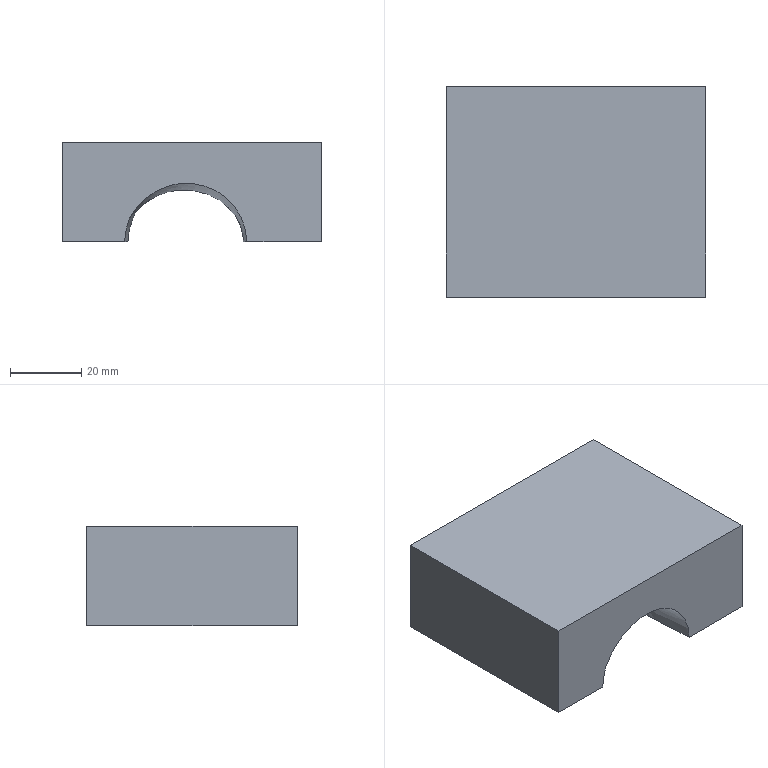NC program | NX | posted with a generic post | part box 72.744 x 59.015 x 27.972 mm
Lines 1 to 1005 of 95982:
N10 G17 G21 G94 G90
(FLOOR_WALL_COPY_1 , TOOL : D63)
N12 T03 M6
N14 G54
N16 G17 G0 G90 X70.872 Y0. S6500 M3
N18 G43 Z30. H3
N20 Z10.025
N22 G94 G1 Z7.025 F1500.
N24 X67.872
N26 X-67.872
N28 X-70.872
N30 Z10.025
N32 G0 Z30.
N34 X70.872
N36 Z9.05
N38 G1 Z6.05
N40 X67.872
N42 X-67.872
N44 X-70.872
N46 Z9.05
N48 G0 Z30.
N50 X70.872
N52 Z8.075
N54 G1 Z5.075
N56 X67.872
N58 X-67.872
N60 X-70.872
N62 Z8.075
N64 G0 Z30.
N66 X70.872
N68 Z7.1
N70 G1 Z4.1
N72 X67.872
N74 X-67.872
N76 X-70.872
N78 Z7.1
N80 G0 Z30.
N82 X70.872
N84 Z6.125
N86 G1 Z3.125
N88 X67.872
N90 X-67.872
N92 X-70.872
N94 Z6.125
N96 G0 Z30.
N98 X70.872
N100 Z5.15
N102 G1 Z2.15
N104 X67.872
N106 X-67.872
N108 X-70.872
N110 Z5.15
N112 G0 Z30.
N114 X70.872
N116 Z4.175
N118 G1 Z1.175
N120 X67.872
N122 X-67.872
N124 X-70.872
N126 Z4.175
N128 G0 Z30.
N130 X70.872
N132 Z3.2
N134 G1 Z0.2
N136 X67.872
N138 X-67.872
N140 X-70.872
N142 Z3.2
N144 G0 Z30.
(FLOOR_WALL_COPY , TOOL : D63)
N146 X70.872
N148 Z3.
N150 G1 Z0.
N152 X67.872
N154 X-67.872
N156 X-70.872
N158 Z3.
N160 G0 Z30.
N162 M5
(DRILLING , TOOL : D6A45)
N164 T01 M6
N166 G54
N168 G17 G0 G90 X-25.98 Y-17.007 S5000 M3
N170 G43 Z30. H1
N172 G94 G81 G98 Z-1. F250. R3.
N174 Y0.
N176 X22.701 Y1.319
N178 X22.872 Y18.771
N180 G80
N182 G0 X22.872 Y18.771 Z30.
N184 M5
(DRILLING_COPY_COPY , TOOL : 4.2ZT)
N186 T13 M6
N188 G54
N190 G17 G0 G90 X-25.98 Y0. S2000 M3
N192 G43 Z30. H13
N194 G94 G83 G98 Z-16.262 F150. Q3. R3.
N196 X22.701 Y1.319
N198 G80
N200 G0 X22.701 Y1.319 Z30.
N202 M5
(DRILLING_COPY_COPY_1 , TOOL : 6.0ZT)
N204 T12 M6
N206 G54
N208 G17 G0 G90 X-25.98 Y-17.007 S2000 M3
N210 G43 Z30. H12
N212 G94 G83 G98 Z-6.803 F150. Q3. R3.
N214 X22.872 Y18.771
N216 G80
N218 G0 X22.872 Y18.771 Z30.
N220 M5
(ZLEVEL_PROFILE , TOOL : D10)
N222 T04 M6
N224 G54
N226 G17 G0 G90 X6.339 Y-35.446 S9500 M3
N228 G43 Z30. H4
N230 Z2.351
N232 G94 G1 Z-0.649 F1000.
N234 X8.783 Y-34.579
N236 G3 X9.432 Y-33.819 R1.
N238 G1 X9.594 Y-32.943 F3000.
N240 X10.353 Y-29.113
N242 G3 X11.174 Y-18.732 R44.736
N244 X10.465 Y-9.092 R135.523
N246 G2 X9.528 Y0.91 R325.209
N248 X9.411 Y14.759 R121.644
N250 X9.859 Y23.223 R452.887
N252 G3 X10.376 Y33.994 R414.056
N254 G1 X10.437 Y35.119
N256 X10.397 Y35.16 Z-1.296
N258 G3 X9.995 Y26.3 R1988.526
N260 X9.326 Y13.99 R418.562
N262 G1 X9.298 Y13.22
N264 G3 X9.504 Y0.141 R115.066
N266 X10.494 Y-9.861 R514.132
N268 G2 X11.135 Y-19.094 R125.7
N270 G1 X11.125 Y-22.179
N272 X11.06 Y-22.941
N274 X11.04 Y-23.711
N276 G2 X10.353 Y-28.93 R42.268
N278 G1 X10.307 Y-29.096
N280 X9.408 Y-33.713
N282 X9.389 Y-33.837
N284 X9.311 Y-33.854 Z-1.939
N286 G2 X10.227 Y-29.204 R167.152
N288 G3 X10.972 Y-23.545 R36.684
N290 X10.881 Y-15.254 R65.015
N292 X10.081 Y-6.784 R218.471
N294 G2 X9.224 Y3.218 R189.269
N296 X9.355 Y17.067 R140.941
N298 G1 X10.072 Y29.378
N300 X10.303 Y34.764
N302 X10.335 Y35.193
N304 X10.293 Y35.197 Z-2.258
N306 X10.242 Y35.201 Z-2.577
N308 X9.894 Y27.839
N310 G3 X9.149 Y15.206 R1037.494
N312 X9.542 Y-2.502 R118.13
N314 X10.353 Y-10.286 R592.303
N316 G2 X10.949 Y-18.325 R129.413
N318 X10.353 Y-28.077 R46.878
N320 G1 X9.202 Y-33.865
N322 X9.078 Y-33.873 Z-3.208
N324 X9.101 Y-33.713
N326 X10.353 Y-27.445
N328 G3 X10.858 Y-19.094 R46.636
N330 X10.247 Y-10.631 R108.014
N332 G2 X9.329 Y-1.836 R626.712
N334 X8.876 Y11.93 R107.709
N336 X9.374 Y21.684 R238.756
N338 G1 X9.408 Y22.453
N340 X9.475 Y23.223
N342 G3 X10.139 Y35.21 R724.458
N344 G1 X10.06 Y35.216 Z-3.519
N346 X9.995 Y35.221 Z-3.831
N348 G2 X9.312 Y23.223 R809.16
N350 G1 X9.256 Y22.453
N352 G3 X8.717 Y12.777 R318.099
N354 X9.068 Y-0.87 R103.127
N356 G1 X9.4 Y-4.476
N358 G2 X10.366 Y-13.394 R340.168
N360 X10.735 Y-20.556 R82.791
N362 X9.905 Y-29.054 R40.595
N364 G1 X8.948 Y-33.713
N366 X8.925 Y-33.876
N368 X8.851 Y-33.877 Z-4.137
N370 X8.765 Z-4.444
N372 X8.939 Y-32.943
N374 X9.732 Y-29.111
N376 G3 X10.573 Y-19.114 R41.802
N378 X10.006 Y-11.4 R104.84
N380 X9.357 Y-5.659 R763.831
N382 G2 X8.546 Y3.218 R176.621
N384 X8.675 Y16.298 R119.75
N386 G1 X8.725 Y17.067
N388 G2 X9.066 Y22.453 R731.199
N390 G1 X9.133 Y23.223
N392 G3 X9.821 Y35.234 R541.045
N394 G1 X9.733 Y35.241 Z-4.743
N396 X9.642 Y35.248 Z-5.043
N398 X9.2 Y27.07
N400 G3 X8.39 Y15.529 R662.276
N402 X8.309 Y3.218 R119.617
N404 X9.364 Y-7.553 R184.128
N406 G2 X10.32 Y-17.555 R149.783
N408 X9.857 Y-27.558 R44.712
N410 G1 X9.712 Y-28.327
N412 X8.57 Y-33.864
N414 X8.468 Y-33.857 Z-5.333
N416 X8.372 Y-33.85 Z-5.623
N418 X9.406 Y-28.901
N420 G3 X10.209 Y-20.64 R38.185
N422 X9.679 Y-12.17 R84.12
N424 G1 X8.767 Y-4.476
N426 X8.666 Y-3.706
N428 X8.571 Y-2.937
N430 X8.506 Y-2.167
N432 X8.263 Y0.455
N434 G2 X7.922 Y8.211 R79.981
N436 X8.46 Y20.145 R147.996
N438 X8.676 Y23.223 R120.911
N440 G1 X8.809 Y24.736
N442 G3 X9.445 Y35.26 R464.927
N444 G1 X9.34 Y35.266 Z-5.907
N446 X9.238 Y35.272 Z-6.192
N448 X8.809 Y28.019
N450 X8.74 Y27.07
N452 G3 X7.848 Y15.529 R583.08
N454 X7.706 Y3.988 R103.887
N456 X8.883 Y-7.553 R148.977
N458 G2 X9.957 Y-18.325 R143.175
N460 X9.453 Y-27.558 R41.597
N462 G1 X9.31 Y-28.327
N464 X8.166 Y-33.713
N466 X8.148 Y-33.831
N468 X8.03 Y-33.823 Z-6.473
N470 X7.902 Y-33.815 Z-6.753
N472 X9.226 Y-27.558
N474 G3 X9.744 Y-19.094 R39.432
N476 X8.807 Y-9.092 R109.813
N478 G2 X7.752 Y-0.629 R274.239
N480 G1 X7.425 Y3.218
N482 G2 X7.536 Y15.529 R107.691
N484 X8.475 Y27.07 R660.147
N486 G3 X9. Y35.286 R752.635
N488 G1 X8.882 Y35.293 Z-7.026
N490 X8.749 Y35.301 Z-7.298
N492 G3 X8.426 Y30.147 R118.708
N494 G1 X8.373 Y29.378
N496 X8.037 Y25.2
N498 G3 X7.112 Y13.99 R282.241
N500 X7.414 Y-0.629 R87.771
N502 G1 X7.511 Y-1.398
N504 X7.587 Y-2.167
N506 X8.855 Y-11.763
N508 G2 X9.52 Y-19.692 R83.246
N510 X8.677 Y-29.036 R37.363
N512 G1 X7.651 Y-33.713
N514 X7.637 Y-33.799
N516 X7.491 Y-33.788 Z-7.559
N518 X7.35 Y-33.778 Z-7.821
N520 X7.36 Y-33.713
N522 X8.714 Y-27.558
N524 X8.809 Y-27.066
N526 G3 X9.163 Y-17.555 R41.263
N528 X7.876 Y-6.784 R161.755
N530 G2 X6.719 Y3.218 R129.688
N532 X7.054 Y18.36 R106.4
N534 G1 X8.085 Y29.378
N536 X8.428 Y34.764
N538 X8.47 Y35.32
N540 X8.353 Y35.327 Z-8.072
N542 X8.201 Y35.337 Z-8.324
N544 G2 X7.265 Y23.864 R343.965
N546 G1 X7.189 Y23.223
N548 G3 X6.295 Y12.425 R168.551
N550 X7.007 Y-3.016 R80.444
N552 G1 X7.767 Y-8.323
N554 X7.884 Y-9.092
N556 G2 X8.968 Y-19.094 R105.46
N558 X8.037 Y-29.437 R35.63
N560 G1 X7.043 Y-33.755
N562 X6.898 Y-33.744 Z-8.567
N564 X6.734 Y-33.732 Z-8.81
N566 X6.913 Y-32.943
N568 X7.821 Y-29.119
N570 G3 X8.675 Y-19.034 R34.177
N572 X7.434 Y-8.323 R105.355
N574 G2 X6.225 Y0.141 R210.374
N576 X6.073 Y15.529 R79.197
N578 X7.265 Y27.102 R385.695
N580 G1 X7.92 Y35.357
N582 X7.783 Y35.367 Z-9.045
N584 X7.615 Y35.379 Z-9.279
N586 G2 X6.493 Y23.391 R246.453
N588 G3 X5.521 Y13.627 R212.909
N590 X5.762 Y0.726 R68.149
N592 G1 X6.004 Y-1.398
N594 X6.957 Y-7.553
N596 X7.353 Y-9.957
N598 G2 X8.391 Y-19.283 R89.956
N600 X7.867 Y-27.558 R34.08
N602 G1 X6.426 Y-33.708
N604 X6.264 Y-33.693 Z-9.504
N606 X6.089 Y-33.677 Z-9.73
N608 X7.405 Y-28.327
N610 G3 X8.092 Y-19.094 R32.734
N612 X6.595 Y-7.553 R105.795
N614 G2 X5.324 Y0.801 R124.203
N616 X5.254 Y15.803 R67.015
N618 G1 X5.64 Y19.376
N620 X6.493 Y26.439
N622 X6.56 Y27.07
N624 X7.322 Y35.4
N626 X7.169 Y35.411 Z-9.945
N628 X7.001 Y35.424 Z-10.161
N630 G2 X5.205 Y19.376 R277.244
N632 G3 X4.544 Y3.988 R79.68
N634 X6.346 Y-8.323 R123.906
N636 G2 X7.784 Y-19.094 R87.154
N638 X7.265 Y-27.595 R32.942
N640 G1 X5.765 Y-33.648
N642 X5.598 Y-33.63 Z-10.368
N644 X5.42 Y-33.611 Z-10.574
N646 X6.946 Y-27.558
N648 X7.102 Y-26.788
N650 G3 X7.367 Y-17.555 R34.192
N652 X5.721 Y-6.993 R115.46
N654 G2 X3.975 Y5.526 R93.648
N656 X4.767 Y19.376 R78.342
N658 G3 X6.684 Y35.449 R255.827
N660 G1 X6.537 Y35.46 Z-10.77
N662 X6.367 Y35.474 Z-10.966
N664 G2 X4.539 Y20.914 R207.585
N666 G3 X3.427 Y7.065 R83.088
N668 X4.964 Y-5.245 R72.463
N670 G2 X7.046 Y-17.555 R127.058
N672 X6.493 Y-28.208 R31.215
N674 G1 X6.247 Y-29.096
N676 X5.085 Y-33.576
N678 X4.924 Y-33.558 Z-11.152
N680 X4.733 Y-33.537 Z-11.338
N682 X6.317 Y-27.558
N684 X6.488 Y-26.788
N686 G3 X6.546 Y-16.017 R34.38
N688 X4.377 Y-4.476 R157.772
N690 G2 X2.879 Y7.835 R67.81
N692 X3.986 Y20.129 R79.387
N694 G3 X6.038 Y35.502 R222.23
N696 G1 X5.888 Y35.515 Z-11.514
N698 X5.727 Y35.529 Z-11.69
N700 G2 X3.528 Y20.145 R220.724
N702 G3 X2.363 Y7.065 R68.177
N704 X4.109 Y-5.245 R65.438
N706 G2 X6.415 Y-17.555 R120.012
N708 X5.999 Y-27.558 R29.773
N710 G1 X5.818 Y-28.327
N712 X4.375 Y-33.498
N714 X4.202 Y-33.478 Z-11.856
N716 X4.02 Y-33.457 Z-12.022
N718 X5.491 Y-28.327
N720 X5.721 Y-27.447
N722 G3 X5.897 Y-16.017 R31.355
N724 X3.406 Y-4.037 R170.523
N726 G2 X2.546 Y17.067 R51.388
N728 G1 X3.917 Y24.971
N730 G3 X5.397 Y35.56 R162.542
N732 G1 X5.248 Y35.574 Z-12.177
N734 X5.084 Y35.59 Z-12.332
N736 G2 X2.573 Y20.145 R174.001
N738 G3 X1.252 Y7.065 R61.632
N740 X3.052 Y-4.476 R61.71
N742 G2 X5.582 Y-16.017 R138.209
N744 X5.553 Y-26.788 R30.899
N746 G1 X5.372 Y-27.558
N748 X3.668 Y-33.413
N750 X3.502 Y-33.391 Z-12.477
N752 X3.33 Y-33.368 Z-12.621
N754 X4.95 Y-28.028
N756 X5.071 Y-27.558
N758 G3 X5.373 Y-16.786 R27.306
N760 X2.804 Y-5.245 R100.196
N762 G2 X0.769 Y5.526 R64.023
N764 X1.948 Y19.376 R49.723
N766 G3 X4.772 Y35.621 R170.733
N768 G1 X4.629 Y35.636 Z-12.755
N770 X4.47 Y35.653 Z-12.889
N772 X3.406 Y28.55
N774 X3.121 Y27.07
N776 X1.309 Y18.606
N778 X0.776 Y15.828
N780 G3 X1.16 Y-0.316 R38.114
N782 G1 X1.98 Y-3.706
N784 G2 X4.95 Y-15.901 R148.998
N786 X4.968 Y-26.788 R29.66
N788 G1 X4.773 Y-27.558
N790 X2.989 Y-33.318
N792 X2.833 Y-33.294 Z-13.011
N794 X2.668 Y-33.268 Z-13.134
N796 X4.487 Y-27.558
N798 X4.682 Y-26.788
N800 G3 X4.665 Y-16.017 R27.403
N802 X1.738 Y-4.476 R110.213
N804 G2 X-0.494 Y7.065 R54.271
N806 X0.972 Y19.376 R44.729
N808 G3 X4.188 Y35.684 R146.131
N810 G1 X4.045 Y35.701 Z-13.246
N812 X3.908 Y35.717 Z-13.357
N814 G2 X0.483 Y19.376 R129.167
N816 G3 X-0.877 Y4.757 R38.621
N818 X1.332 Y-4.476 R59.136
N820 G2 X4.508 Y-16.786 R96.652
N822 X4.225 Y-27.558 R24.937
N824 G1 X3.987 Y-28.327
N826 X2.358 Y-33.215
N828 X2.213 Y-33.189 Z-13.458
N830 X2.069 Y-33.164 Z-13.558
N832 X3.967 Y-27.558
N834 X4.181 Y-26.788
N836 G3 X4.178 Y-16.291 R26.3
N838 X1.09 Y-4.962 R94.501
N840 G1 X-0.194 Y-0.823
N842 G2 X-1.741 Y9.373 R34.478
N844 X0.318 Y20.526 R51.448
N846 G3 X3.651 Y35.748 R107.634
N848 X3.279 Y36.676 R1.
N850 G1 X1.293 Y38.24
N852 Z-10.558
N854 G0 Z30.
N856 X-12.168 Y38.156
N858 Z2.351
N860 G1 Z-0.649 F1000.
N862 X-14.167 Y36.537
N864 G3 X-14.526 Y35.603 R1.
N866 G2 X-13.502 Y28.608 R296.97 F3000.
N868 X-13.329 Y7.835 R83.197
N870 G3 X-13.417 Y4.757 R14.398
N872 G2 X-15.223 Y-18.596 R84.348
N874 G3 X-15.284 Y-19.199 R2.628
N876 X-14.237 Y-29.096 R55.047
N878 G1 X-13.309 Y-33.816
N880 X-13.255 Y-33.839 Z-1.296
N882 X-13.876 Y-30.635
N884 X-14.035 Y-29.866
N886 G2 X-15.247 Y-19.094 R56.765
N888 G1 X-15.209 Y-18.707
N890 G3 X-13.324 Y3.988 R83.761
N892 G1 X-13.381 Y4.988
N894 G2 X-13.265 Y8.162 R17.013
N896 G3 X-12.983 Y10.856 R53.59
N898 X-13.266 Y27.07 R83.968
N900 X-14.495 Y35.622 R278.481
N902 G1 X-14.442 Y35.647 Z-1.939
N904 G2 X-13.431 Y28.889 R301.166
N906 X-13.26 Y7.435 R83.172
N908 G3 X-13.32 Y5.203 R11.819
N910 G2 X-15.12 Y-18.616 R83.665
N912 G3 X-15.178 Y-19.181 R2.433
N914 X-14.13 Y-29.063 R55.059
N916 G1 X-13.178 Y-33.857
N918 X-13.087 Y-33.869 Z-2.577
N920 X-13.11 Y-33.713
N922 X-14.049 Y-29.013
N924 G2 X-15.081 Y-19.178 R53.468
N926 X-15.017 Y-18.567 R2.664
N928 G3 X-13.158 Y3.988 R82.976
N930 G1 X-13.219 Y5.106
N932 G2 X-13.134 Y7.763 R15.413
N934 G3 X-13.308 Y28.608 R82.477
N936 X-14.37 Y35.675 R236.416
N938 G1 X-14.25 Y35.637 Z-3.208
N940 G2 X-13.271 Y29.167 R366.336
N942 X-12.917 Y8.604 R83.095
N944 G1 X-13.088 Y7.065
N946 G3 X-13.125 Y5.526 R8.739
N948 G2 X-14.921 Y-18.594 R82.052
N950 G3 X-14.974 Y-19.075 R2.154
N952 X-13.91 Y-29.096 R49.119
N954 G1 X-12.955 Y-33.877
N956 X-12.887 Y-33.88 Z-3.519
N958 X-12.812 Y-33.883 Z-3.831
N960 X-12.841 Y-33.713
N962 X-13.761 Y-29.096
N964 X-13.939 Y-28.327
N966 G2 X-14.849 Y-19.257 R55.662
N968 X-14.776 Y-18.544 R2.987
N970 G3 X-12.883 Y3.988 R81.829
N972 G1 X-12.97 Y5.526
N974 G2 X-12.874 Y7.835 R13.275
N976 G3 X-13.058 Y28.608 R82.135
N978 X-14.125 Y35.582 R267.853
N980 G1 X-13.952 Y35.538 Z-4.444
N982 G2 X-12.822 Y27.91 R240.627
N984 X-12.749 Y7.642 R79.674
N986 G3 X-12.819 Y5.526 R11.621
N988 G2 X-14.656 Y-18.691 R81.455
N990 G1 X-14.717 Y-19.094
N992 X-14.686 Y-19.864
N994 X-14.582 Y-22.172
N996 X-14.497 Y-22.941
N998 X-14.482 Y-23.149
N1000 G3 X-13.756 Y-28.421 R41.633
N1002 G1 X-12.645 Y-33.876
N1004 X-12.554 Y-33.871 Z-4.743
N1006 X-12.467 Y-33.866 Z-5.043
N1008 X-12.491 Y-33.713
N1010 X-13.507 Y-28.788
N1012 G2 X-14.479 Y-20.619 R48.434
N1014 G1 X-14.519 Y-19.425
N1016 G2 X-14.419 Y-18.376 R4.114
N1018 G3 X-12.583 Y4.757 R80.753
N1020 G1 X-12.628 Y5.526
N1022 G2 X-12.549 Y7.835 R11.821
N1024 G3 X-12.629 Y27.839 R82.372
N1026 G2 X-13.613 Y35.294 R160.842
N1028 G1 X-13.453 Y35.283 Z-5.333
N1030 X-13.29 Y35.272 Z-5.623
N1032 X-12.999 Y31.686
N1034 X-12.896 Y30.917
N1036 X-12.452 Y27.839
N1038 X-12.36 Y27.07
N1040 G2 X-12.371 Y7.835 R79.771
N1042 G3 X-12.44 Y5.526 R11.863
N1044 G2 X-14.348 Y-18.821 R79.515
N1046 G3 X-13.559 Y-27.558 R53.953
N1048 G1 X-12.258 Y-33.852
N1050 X-12.143 Y-33.842 Z-5.907
N1052 X-12.025 Y-33.833 Z-6.192
N1054 X-13.166 Y-28.425
N1056 G2 X-14.049 Y-21.399 R42.692
N1058 G1 X-14.156 Y-18.848
N1060 G3 X-12.221 Y5.526 R79.349
N1062 G2 X-12.167 Y7.835 R10.804
N1064 G3 X-12.597 Y30.147 R79.745
N1066 G1 X-12.669 Y30.917
N1068 X-12.976 Y35.285
N1070 X-12.817 Y35.291 Z-6.473
N1072 X-12.664 Y35.298 Z-6.753
N1074 X-12.622 Y34.764
N1076 X-12.336 Y30.147
N1078 X-12.261 Y29.378
N1080 G2 X-11.958 Y7.835 R78.674
N1082 G3 X-11.997 Y5.526 R11.438
N1084 G2 X-13.576 Y-17.227 R76.997
N1086 G1 X-13.902 Y-18.681
N1088 X-13.92 Y-18.874
N1090 G3 X-12.832 Y-28.914 R48.229
N1092 G1 X-11.772 Y-33.818
N1094 X-11.641 Y-33.81 Z-7.026
N1096 X-11.506 Y-33.801 Z-7.298
N1098 X-11.52 Y-33.713
N1100 X-12.804 Y-27.879
N1102 G2 X-13.689 Y-18.704 R49.902
N1104 G3 X-12.032 Y-9.369 R73.392
N1106 X-11.755 Y5.526 R72.103
N1108 G2 X-11.473 Y10.143 R71.719
N1110 G3 X-11.13 Y18.606 R85.202
N1112 X-11.912 Y28.608 R85.687
N1114 G1 X-12.36 Y35.31
N1116 X-12.211 Y35.317 Z-7.559
N1118 X-12.069 Y35.323 Z-7.821
N1120 X-11.532 Y27.839
N1122 X-11.465 Y27.07
N1124 X-11.243 Y24.815
N1126 G2 X-10.932 Y15.027 R73.707
N1128 G1 X-10.994 Y13.22
N1130 X-11.443 Y4.907
N1132 X-11.442 Y4.757
N1134 G2 X-13.442 Y-18.645 R76.004
N1136 G1 X-13.421 Y-19.094
N1138 X-13.359 Y-20.936
N1140 G3 X-12.259 Y-29.145 R41.6
N1142 G2 X-11.231 Y-33.781 R161.339
N1144 G1 X-11.083 Y-33.769 Z-8.072
N1146 X-10.922 Y-33.756 Z-8.324
N1148 X-11.803 Y-29.866
N1150 X-11.882 Y-29.551
N1152 G2 X-13.111 Y-20.541 R41.394
N1154 G1 X-13.148 Y-19.094
N1156 X-13.164 Y-18.677
N1158 X-13.112 Y-18.325
N1160 X-12.786 Y-16.855
N1162 G3 X-11.129 Y3.988 R75.557
N1164 X-10.742 Y21.684 R132.674
N1166 X-11.768 Y35.355 R1114.465
N1168 G1 X-11.63 Y35.371 Z-8.567
N1170 X-11.474 Y35.39 Z-8.81
N1172 G3 X-10.678 Y26.3 R1104.06
N1174 G2 X-10.815 Y3.218 R121.382
N1176 X-12.88 Y-18.325 R75.214
N1178 G3 X-11.748 Y-28.92 R43.315
N1180 G1 X-10.622 Y-33.731
N1182 X-10.472 Y-33.718 Z-9.045
N1184 X-10.311 Y-33.704 Z-9.279
N1186 X-11.501 Y-28.709
N1188 G2 X-12.549 Y-20.675 R38.964
N1190 G1 X-12.609 Y-18.325
N1192 X-12.549 Y-17.988
N1194 G3 X-10.474 Y-0.19 R73.57
N1196 G1 X-10.49 Y2.449
N1198 G3 X-10.101 Y23.992 R108.574
N1200 G1 X-10.221 Y25.531
N1202 X-11.176 Y35.424
N1204 X-11.024 Y35.442 Z-9.504
N1206 X-10.85 Y35.462 Z-9.73
N1208 X-9.83 Y25.531
N1210 G2 X-10.084 Y2.015 R103.008
N1212 G3 X-10.187 Y0.251 R13.157
N1214 G2 X-12.29 Y-17.935 R73.854
N1216 G3 X-11.295 Y-28.327 R42.45
N1218 G1 X-9.987 Y-33.672
N1220 X-9.829 Y-33.656 Z-9.945
N1222 X-9.666 Y-33.64 Z-10.161
N1224 X-10.974 Y-28.327
N1226 G2 X-11.997 Y-19.094 R38.829
N1228 X-11.873 Y-17.232 R5.344
N1230 G1 X-11.763 Y-16.786
N1232 G3 X-9.995 Y-3.908 R73.119
N1234 X-9.891 Y0.141 R92.621
N1236 X-9.206 Y23.223 R98.449
N1238 X-10.537 Y35.498 R636.712
N1240 G1 X-10.377 Y35.516 Z-10.368
N1242 X-10.215 Y35.534 Z-10.574
N1244 X-9.095 Y26.3
N1246 X-8.765 Y23.091
N1248 G2 X-9.573 Y-0.629 R87.193
N1250 G3 X-9.713 Y-3.581 R317.09
N1252 G2 X-11.689 Y-17.555 R72.48
N1254 G3 X-11.276 Y-25.249 R48.498
N1256 X-10.5 Y-28.954 R41.757
N1258 G1 X-9.304 Y-33.608
N1260 X-9.136 Y-33.593 Z-10.77
N1262 X-8.958 Y-33.577 Z-10.966
N1264 X-10.488 Y-27.736
N1266 G2 X-11.365 Y-17.201 R40.276
N1268 G3 X-9.758 Y-7.794 R68.528
N1270 X-9.355 Y-2.167 R100.065
N1272 X-8.323 Y23.223 R84.73
N1274 G1 X-8.495 Y24.761
N1276 X-9.881 Y35.571
N1278 X-9.72 Y35.589 Z-11.152
N1280 X-9.548 Y35.608 Z-11.338
N1282 X-8.061 Y24.761
N1284 X-7.796 Y22.453
N1286 G2 X-8.499 Y0.141 R75.903
N1288 G1 X-8.62 Y-0.629
N1290 X-8.987 Y-2.529
N1292 G3 X-9.22 Y-4.411 R14.016
N1294 G2 X-11.023 Y-16.786 R70.105
N1296 G3 X-9.716 Y-29.439 R37.484
N1298 G1 X-9.596 Y-29.866
N1300 X-9.385 Y-30.635
N1302 X-8.596 Y-33.539
N1304 X-8.432 Y-33.522 Z-11.514
N1306 X-8.25 Y-33.502 Z-11.69
N1308 X-9.469 Y-29.096
N1310 X-9.716 Y-28.267
N1312 G2 X-10.607 Y-16.017 R35.54
N1314 G3 X-9.229 Y-7.605 R65.078
N1316 G1 X-9. Y-5.245
N1318 X-8.944 Y-4.74
N1320 X-8.159 Y-0.629
N1322 X-7.723 Y1.882
N1324 G3 X-7.222 Y21.389 R67.043
N1326 G1 X-7.63 Y24.761
N1328 X-9.217 Y35.645
N1330 X-9.055 Y35.663 Z-11.856
N1332 X-8.897 Y35.681 Z-12.022
N1334 X-7.084 Y23.992
N1336 X-6.66 Y20.591
N1338 G2 X-7.376 Y0.991 R61.351
N1340 G1 X-8.775 Y-6.014
N1342 G2 X-10.335 Y-16.017 R98.084
N1344 G3 X-9.716 Y-26.988 R37.429
N1346 G1 X-7.893 Y-33.459
N1348 X-7.726 Y-33.437 Z-12.177
N1350 X-7.549 Y-33.415 Z-12.332
N1352 X-9.256 Y-27.558
N1354 X-9.447 Y-26.788
N1356 G2 X-9.945 Y-15.247 R37.022
N1358 G3 X-8.684 Y-7.553 R114.997
N1360 G1 X-8.543 Y-6.784
N1362 X-7.176 Y-0.629
N1364 X-6.69 Y1.83
N1366 G3 X-6.098 Y19.979 R56.196
N1368 G1 X-6.521 Y23.223
N1370 X-8.562 Y35.719
N1372 X-8.403 Y35.737 Z-12.477
N1374 X-8.246 Y35.755 Z-12.621
N1376 X-6.06 Y23.223
N1378 X-5.584 Y19.765
N1380 G2 X-6.74 Y-0.867 R53.944
N1382 G3 X-9.408 Y-13.708 R149.58
N1384 X-9.147 Y-26.788 R35.566
N1386 G1 X-8.962 Y-27.558
N1388 X-7.206 Y-33.367
N1390 X-7.038 Y-33.342 Z-12.755
N1392 X-6.871 Y-33.317 Z-12.889
N1394 X-8.656 Y-27.558
N1396 X-8.861 Y-26.788
N1398 G2 X-9.221 Y-14.478 R35.054
N1400 X-6.241 Y-0.813 R119.511
N1402 G3 X-4.986 Y18.943 R47.529
N1404 G1 X-5.617 Y23.223
N1406 X-7.606 Y33.994
N1408 X-7.93 Y35.793
N1410 X-7.784 Y35.81 Z-13.011
N1412 X-7.633 Y35.829 Z-13.134
N1414 G2 X-4.622 Y20.018 R3728.251
N1416 X-5.345 Y0.711 R43.579
N1418 G1 X-7.124 Y-5.946
N1420 G3 X-8.955 Y-14.745 R80.656
N1422 X-8.741 Y-26.019 R33.611
N1424 X-6.556 Y-33.267 R78.335
N1426 G1 X-6.405 Y-33.24 Z-13.246
N1428 X-6.251 Y-33.212 Z-13.357
N1430 X-7.401 Y-29.769
N1432 X-8.056 Y-27.68
N1434 G2 X-8.953 Y-22.951 R20.676
N1436 X-8.172 Y-11.871 R39.47
N1438 X-5.207 Y-0.629 R147.134
N1440 G3 X-4.037 Y19.376 R40.93
N1442 G1 X-6.988 Y33.994
N1444 X-7.356 Y35.863
N1446 X-7.225 Y35.881 Z-13.458
N1448 X-7.091 Y35.899 Z-13.558
N1450 X-6.629 Y33.554
N1452 X-3.435 Y18.811
N1454 G2 X-3.54 Y3.715 R34.553
N1456 G1 X-3.832 Y2.449
N1458 X-6.816 Y-7.553
N1460 G3 X-8.749 Y-17.886 R55.644
N1462 X-7.467 Y-28.74 R26.467
N1464 G1 X-5.974 Y-33.163
N1466 X-5.843 Y-33.137 Z-13.648
N1468 X-5.703 Y-33.11 Z-13.738
N1470 X-7.401 Y-28.243
N1472 X-7.615 Y-27.558
N1474 G2 X-8.215 Y-15.247 R28.015
N1476 X-4.519 Y-1.398 R79.791
N1478 G3 X-2.299 Y7.434 R43.424
N1480 X-0.115 Y-2.512 R38.112
N1482 G2 X3.707 Y-15.247 R113.623
N1484 X4.11 Y-26.019 R26.494
N1486 X1.805 Y-33.114 R61.292
N1488 G1 X1.659 Y-33.083 Z-13.826
N1490 X1.522 Y-33.052 Z-13.914
N1492 X3.498 Y-27.558
N1494 X3.711 Y-26.788
N1496 G3 X3.772 Y-16.786 R23.497
N1498 X0.318 Y-5.025 R69.677
N1500 G2 X-2.382 Y3.694 R70.435
N1502 G1 X-2.736 Y2.449
N1504 X-5.857 Y-6.585
N1506 G3 X-8.36 Y-19.094 R49.598
N1508 X-6.847 Y-29.096 R24.208
N1510 G1 X-5.413 Y-33.048
N1512 X-5.271 Y-33.018 Z-14.001
N1514 X-5.123 Y-32.987 Z-14.087
N1516 X-6.806 Y-28.561
N1518 G2 X-8.065 Y-22.707 R19.806
N1520 X-6.629 Y-10.315 R35.748
N1522 X-2.476 Y1.364 R132.933
N1524 G1 X0.88 Y-7.553
N1526 G2 X3.663 Y-17.555 R57.291
N1528 X3.481 Y-26.788 R22.669
N1530 G1 X3.252 Y-27.558
N1532 X1.24 Y-32.991
N1534 X1.099 Y-32.957 Z-14.174
N1536 X0.947 Y-32.92 Z-14.261
N1538 X2.994 Y-27.558
N1540 X3.231 Y-26.788
N1542 G3 X3.165 Y-16.215 R23.264
N1544 X-0.775 Y-4.371 R72.939
N1546 G1 X-2.509 Y-0.348
N1548 G3 X-6.985 Y-12.939 R71.232
N1550 X-7.495 Y-25.249 R29.801
N1552 X-4.816 Y-32.915 R47.087
N1554 G1 X-4.661 Y-32.876 Z-14.349
N1556 X-4.499 Y-32.835 Z-14.436
N1558 X-5.92 Y-29.439
N1560 G2 X-7.501 Y-17.447 R23.08
N1562 X-2.502 Y-1.973 R45.804
N1564 X3.002 Y-16.786 R60.231
N1566 X2.969 Y-26.788 R21.531
N1568 G1 X2.634 Y-27.839
N1570 X0.918 Y-32.174
N1572 X0.633 Y-32.834
N1574 X0.483 Y-32.792 Z-14.525
N1576 X0.31 Y-32.744 Z-14.613
N1578 X0.557 Y-32.174
N1580 X2.45 Y-27.558
N1582 X2.704 Y-26.788
N1584 G3 X2.876 Y-17.555 R20.413
N1586 X-2.491 Y-3.336 R48.881
N1588 X-7.401 Y-19.568 R37.6
N1590 X-5.733 Y-29.096 R20.774
N1592 G1 X-4.313 Y-32.442
N1594 X-4.168 Y-32.744
N1596 X-3.998 Y-32.691 Z-14.701
N1598 X-3.823 Y-32.636 Z-14.789
N1600 X-4.04 Y-32.174
N1602 X-5.408 Y-29.096
N1604 G2 X-7.161 Y-20.633 R19.329
N1606 X-2.483 Y-4.581 R32.792
N1608 X2.528 Y-17.203 R42.318
N1610 X2.634 Y-25.967 R21.571
N1612 X-0.046 Y-32.632 R39.521
N1614 G1 X-0.229 Y-32.574 Z-14.876
N1616 X-0.414 Y-32.514 Z-14.964
N1618 G3 X2.517 Y-25.249 R31.013
N1620 X2.129 Y-16.786 R21.031
N1622 G1 X1.944 Y-16.017
N1624 G3 X-2.489 Y-5.828 R34.246
N1626 X-6.858 Y-22.034 R28.69
N1628 X-5.18 Y-28.922 R17.386
N1630 G1 X-3.541 Y-32.366
N1632 X-3.465 Y-32.516
N1634 X-3.27 Y-32.434 Z-15.052
N1636 X-3.077 Y-32.353 Z-15.14
N1638 X-4.712 Y-29.096
N1640 G2 X-6.505 Y-22.941 R16.573
N1642 X-2.483 Y-6.995 R25.686
N1644 X2.411 Y-20.259 R29.149
N1646 X1.531 Y-27.558 R16.235
N1648 G1 X-0.454 Y-31.738
N1650 X-0.8 Y-32.351
N1652 X-0.999 Y-32.263 Z-15.228
N1654 X-1.212 Y-32.169 Z-15.316
N1656 G3 X1.923 Y-25.249 R25.455
N1658 X1.475 Y-16.786 R19.503
N1660 G1 X1.261 Y-16.017
N1662 G3 X-2.467 Y-8.042 R25.492
N1664 X-5.84 Y-25.249 R23.275
N1666 X-2.668 Y-32.174 R28.177
N1668 X-1.782 Y-32.638 R1.
N1670 G1 X-1.937 Y-27.179
N1672 Z-12.316
N1674 G0 Z30.
N1676 X-1.555 Y-18.296
N1678 Z-12.492
N1680 G1 Z-15.492 F1000.
N1682 X1.231 Y-19.624
N1684 G2 X1.797 Y-20.448 R1.
N1686 X1.593 Y-25.249 R19.875 F3000.
N1688 X-1.639 Y-31.915 R21.543
N1690 X-2.253 Y-31.913 R-0.311
N1692 X-5.505 Y-25.249 R23.663
N1694 X-2.459 Y-9.1 R21.422
N1696 X0.318 Y-14.338 R20.416
N1698 X1.797 Y-20.448 R19.875
N1700 G1 X1.645 Y-20.462 Z-15.581
N1702 X1.447 Y-20.481 Z-15.67
N1704 G3 X-2.443 Y-10.182 R20.886
N1706 X-5.169 Y-25.249 R19.728
N1708 X-1.961 Y-31.443 R20.96
N1710 X1.502 Y-23.711 R15.592
N1712 X1.447 Y-20.481 R20.886
N1714 G1 X1.309 Y-20.496 Z-15.758
N1716 X1.136 Y-20.516 Z-15.846
N1718 X1.149 Y-20.633
N1720 G2 X-1.997 Y-30.516 R12.308
N1722 X-4.993 Y-24.48 R15.972
N1724 X-2.418 Y-11.258 R18.118
N1726 X1.09 Y-20.104 R19.492
N1728 G1 X1.136 Y-20.516
N1730 X0.952 Y-20.536 Z-15.935
N1732 X0.764 Y-20.558 Z-16.025
N1734 G3 X-2.386 Y-12.353 R17.533
N1736 X-4.415 Y-25.249 R16.258
N1738 X-1.997 Y-29.62 R14.16
N1740 X0.861 Y-21.816 R10.866
N1742 X0.764 Y-20.558 R17.533
N1744 G1 X0.57 Y-20.582 Z-16.115
N1746 X0.377 Y-20.605 Z-16.204
N1748 G2 X0.482 Y-21.893 R15.926
N1750 X-1.964 Y-28.769 R9.778
N1752 X-3.987 Y-25.249 R8.486
N1754 X-2.36 Y-13.444 R14.712
N1756 X0.377 Y-20.605 R15.926
N1758 G1 X0.173 Y-20.631 Z-16.292
N1760 X-0.034 Y-20.657 Z-16.379
N1762 G3 X-2.329 Y-14.562 R14.063
N1764 X-3.783 Y-24.48 R13.432
N1766 X-1.964 Y-27.899 R7.834
N1768 X0.077 Y-22.566 R8.195
N1770 X-0.034 Y-20.657 R14.063
N1772 G1 X-0.256 Y-20.687 Z-16.468
N1774 X-0.468 Y-20.715 Z-16.557
N1776 G2 X-0.376 Y-21.784 R11.761
N1778 G1 X-0.35 Y-22.448
N1780 G2 X-1.963 Y-27.026 R6.563
N1782 X-3.046 Y-25.249 R5.37
N1784 X-2.287 Y-15.814 R11.4
N1786 X-0.468 Y-20.715 R11.761
N1788 G1 X-0.719 Y-20.749 Z-16.646
N1790 X-0.971 Y-20.783 Z-16.735
N1792 X-0.991 Y-20.633
N1794 G3 X-2.248 Y-17.07 R9.606
N1796 X-2.769 Y-24.61 R10.41
N1798 G1 X-2.048 Y-26.019
N1800 X-1.922 Y-26.124
N1802 G3 X-0.886 Y-21.402 R6.916
N1804 G1 X-0.971 Y-20.783
N1806 X-1.081 Y-21.117 Z-16.794
N1808 X-1.234 Y-21.455 Z-16.853
N1810 X-1.376 Y-21.791 Z-16.912
N1812 G2 X-1.958 Y-25.088 R8.021
N1814 X-2.19 Y-18.544 R8.56
N1816 X-1.376 Y-21.791 R8.021
N1818 X-1.845 Y-22.674 R1.
N1820 G1 Z-13.912
N1822 G0 Z30.
N1824 X-4.636 Y38.601
N1826 Z-10.738
N1828 G1 Z-13.738 F1000.
N1830 X-6.542 Y36.884
N1832 G3 X-6.85 Y35.933 R1.
N1834 X-3.263 Y20.145 R595.928 F3000.
N1836 G2 X-2.131 Y12.057 R43.469
N1838 X0.296 Y22. R84.07
N1840 G3 X3.412 Y35.777 R90.933
N1842 G1 X3.29 Y35.794 Z-13.826
N1844 X3.168 Y35.81 Z-13.914
N1846 X1.862 Y28.956
N1848 X1.585 Y27.839
N1850 X1.189 Y26.3
N1852 X-1.412 Y17.837
N1854 X-1.934 Y16.189
N1856 X-2.765 Y20.145
N1858 G2 X-6.609 Y35.967 R335.733
N1860 G1 X-6.486 Y35.987 Z-14.001
N1862 X-6.357 Y36.008 Z-14.087
N1864 G3 X-1.824 Y18.388 R349.942
N1866 X2.918 Y35.845 R90.309
N1868 G1 X2.792 Y35.862 Z-14.174
N1870 X2.665 Y35.88 Z-14.261
N1872 G2 X-1.735 Y20.432 R68.529
N1874 X-6.1 Y36.052 R162.524
N1876 G1 X-5.972 Y36.074 Z-14.349
N1878 X-5.836 Y36.098 Z-14.436
N1880 G3 X-1.671 Y22.055 R121.085
N1882 X2.391 Y35.923 R59.964
N1884 G1 X2.249 Y35.945 Z-14.525
N1886 X2.106 Y35.968 Z-14.613
N1888 G2 X-1.615 Y23.635 R52.615
N1890 X-5.553 Y36.165 R85.642
N1892 G1 X-5.418 Y36.198 Z-14.701
N1894 X-5.269 Y36.233 Z-14.789
N1896 G3 X-1.572 Y25.089 R68.545
N1898 X1.816 Y36.016 R47.524
N1900 G1 X1.659 Y36.046 Z-14.876
N1902 X1.498 Y36.076 Z-14.964
N1904 G2 X-1.542 Y26.444 R44.289
N1906 X-4.973 Y36.3 R58.809
N1908 G1 X-4.814 Y36.332 Z-15.052
N1910 X-4.653 Y36.364 Z-15.14
N1912 G3 X-1.521 Y27.796 R49.135
N1914 X1.177 Y36.138 R41.778
N1916 G1 X1.011 Y36.174 Z-15.228
N1918 X0.831 Y36.213 Z-15.316
N1920 G2 X-1.525 Y29.11 R40.778
N1922 X-4.325 Y36.431 R48.214
N1924 G1 X-4.144 Y36.474 Z-15.404
N1926 X-3.954 Y36.518 Z-15.492
N1928 X-1.813 Y30.917
N1930 X-1.547 Y30.396
N1932 X-1.226 Y31.091
N1934 X0.475 Y36.294
N1936 X0.288 Y36.344 Z-15.581
N1938 X0.091 Y36.397 Z-15.67
N1940 X-1.575 Y31.72
N1942 X-3.562 Y36.614
N1944 X-3.356 Y36.676 Z-15.758
N1946 X-3.144 Y36.739 Z-15.846
N1948 X-1.607 Y33.137
N1950 X-0.307 Y36.51
N1952 X-0.534 Y36.588 Z-15.935
N1954 X-0.75 Y36.663 Z-16.025
N1956 X-1.509 Y34.764
N1958 X-1.635 Y34.498
N1960 X-2.7 Y36.88
N1962 X-2.472 Y36.969 Z-16.115
N1964 X-2.227 Y37.064 Z-16.204
N1966 X-1.662 Y35.851
N1968 X-1.222 Y36.839
N1970 G3 X-1.327 Y37.834 R1.
N1972 G1 X-1.676 Y41.133
N1974 Z-13.204
N1976 G0 Z30.
N1978 M5